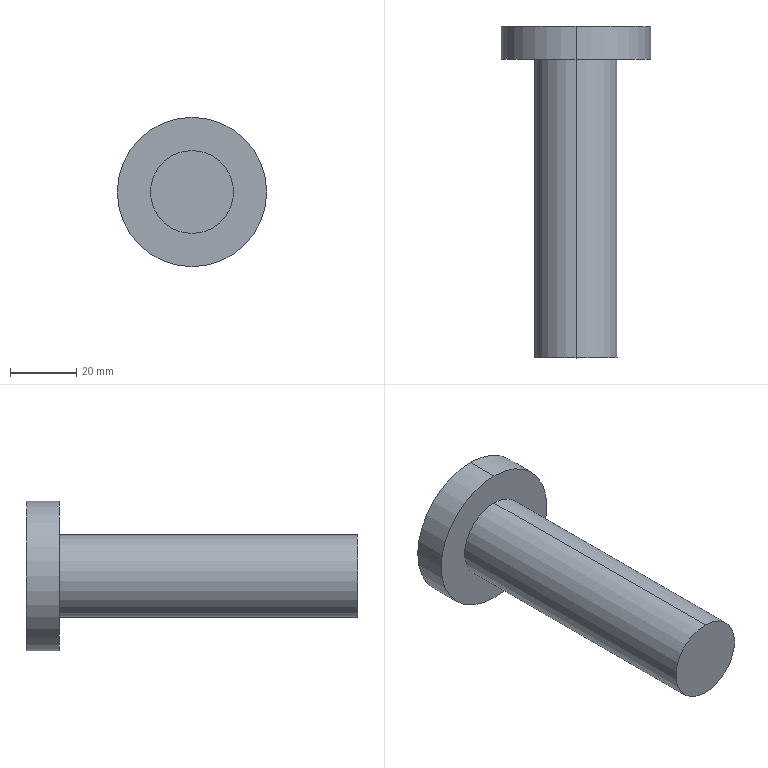Part | SolidWorks | features Extrusion 1, ICE 1 | 1 solid | 7 faces | box 45 x 100 x 45 mm | volume 60083 mm3 | cylinder 4 | plane 3 | commonest cylinder face diameters 25 x2 45 x2
STEP:
#1=CARTESIAN_POINT('',(0.,90.,22.5));
#2=VERTEX_POINT('',#1);
#3=CARTESIAN_POINT('',(0.,90.,-22.5));
#4=VERTEX_POINT('',#3);
#5=CARTESIAN_POINT('',(0.,90.,0.));
#6=DIRECTION('',(0.,1.,0.));
#7=DIRECTION('',(0.,0.,1.));
#8=AXIS2_PLACEMENT_3D('',#5,#6,#7);
#9=CIRCLE('',#8,22.5);
#10=EDGE_CURVE('',#2,#4,#9,.T.);
#11=ORIENTED_EDGE('',*,*,#10,.T.);
#12=CARTESIAN_POINT('',(0.,100.,-22.5));
#13=VERTEX_POINT('',#12);
#14=CARTESIAN_POINT('',(0.,90.,-22.5));
#15=DIRECTION('',(0.,1.,0.));
#16=VECTOR('',#15,1000.);
#17=LINE('',#14,#16);
#18=EDGE_CURVE('',#4,#13,#17,.T.);
#19=ORIENTED_EDGE('',*,*,#18,.T.);
#20=CARTESIAN_POINT('',(0.,100.,22.5));
#21=VERTEX_POINT('',#20);
#22=CARTESIAN_POINT('',(0.,100.,0.));
#23=DIRECTION('',(0.,1.,0.));
#24=DIRECTION('',(0.,0.,1.));
#25=AXIS2_PLACEMENT_3D('',#22,#23,#24);
#26=CIRCLE('',#25,22.5);
#27=EDGE_CURVE('',#21,#13,#26,.T.);
#28=ORIENTED_EDGE('',*,*,#27,.F.);
#29=CARTESIAN_POINT('',(0.,90.,22.5));
#30=DIRECTION('',(0.,1.,0.));
#31=VECTOR('',#30,1000.);
#32=LINE('',#29,#31);
#33=EDGE_CURVE('',#2,#21,#32,.T.);
#34=ORIENTED_EDGE('',*,*,#33,.F.);
#35=EDGE_LOOP('',(#11,#19,#28,#34));
#36=FACE_OUTER_BOUND('',#35,.T.);
#37=CARTESIAN_POINT('',(0.,90.,0.));
#38=DIRECTION('',(0.,1.,0.));
#39=DIRECTION('',(0.,0.,1.));
#40=AXIS2_PLACEMENT_3D('',#37,#38,#39);
#41=CYLINDRICAL_SURFACE('',#40,22.5);
#42=ADVANCED_FACE('',(#36),#41,.T.);
#43=CARTESIAN_POINT('',(0.,90.,12.5));
#44=VERTEX_POINT('',#43);
#45=CARTESIAN_POINT('',(0.,90.,-12.5));
#46=VERTEX_POINT('',#45);
#47=CARTESIAN_POINT('',(0.,90.,0.));
#48=DIRECTION('',(0.,1.,0.));
#49=DIRECTION('',(0.,0.,1.));
#50=AXIS2_PLACEMENT_3D('',#47,#48,#49);
#51=CIRCLE('',#50,12.5);
#52=EDGE_CURVE('',#44,#46,#51,.T.);
#53=ORIENTED_EDGE('',*,*,#52,.F.);
#54=CARTESIAN_POINT('',(0.,0.,12.5));
#55=VERTEX_POINT('',#54);
#56=CARTESIAN_POINT('',(0.,100.,12.5));
#57=DIRECTION('',(0.,-1.,0.));
#58=VECTOR('',#57,1000.);
#59=LINE('',#56,#58);
#60=EDGE_CURVE('',#44,#55,#59,.T.);
#61=ORIENTED_EDGE('',*,*,#60,.T.);
#62=CARTESIAN_POINT('',(0.,0.,-12.5));
#63=VERTEX_POINT('',#62);
#64=CARTESIAN_POINT('',(0.,0.,0.));
#65=DIRECTION('',(0.,1.,0.));
#66=DIRECTION('',(0.,0.,1.));
#67=AXIS2_PLACEMENT_3D('',#64,#65,#66);
#68=CIRCLE('',#67,12.5);
#69=EDGE_CURVE('',#55,#63,#68,.T.);
#70=ORIENTED_EDGE('',*,*,#69,.T.);
#71=CARTESIAN_POINT('',(0.,100.,-12.5));
#72=DIRECTION('',(0.,-1.,0.));
#73=VECTOR('',#72,1000.);
#74=LINE('',#71,#73);
#75=EDGE_CURVE('',#46,#63,#74,.T.);
#76=ORIENTED_EDGE('',*,*,#75,.F.);
#77=EDGE_LOOP('',(#53,#61,#70,#76));
#78=FACE_OUTER_BOUND('',#77,.T.);
#79=CARTESIAN_POINT('',(0.,100.,0.));
#80=DIRECTION('',(0.,-1.,0.));
#81=DIRECTION('',(0.,0.,-1.));
#82=AXIS2_PLACEMENT_3D('',#79,#80,#81);
#83=CYLINDRICAL_SURFACE('',#82,12.5);
#84=ADVANCED_FACE('',(#78),#83,.T.);
#85=ORIENTED_EDGE('',*,*,#60,.F.);
#86=CARTESIAN_POINT('',(0.,90.,0.));
#87=DIRECTION('',(0.,1.,0.));
#88=DIRECTION('',(0.,0.,1.));
#89=AXIS2_PLACEMENT_3D('',#86,#87,#88);
#90=CIRCLE('',#89,12.5);
#91=EDGE_CURVE('',#46,#44,#90,.T.);
#92=ORIENTED_EDGE('',*,*,#91,.F.);
#93=ORIENTED_EDGE('',*,*,#75,.T.);
#94=CARTESIAN_POINT('',(0.,0.,0.));
#95=DIRECTION('',(0.,1.,0.));
#96=DIRECTION('',(0.,0.,1.));
#97=AXIS2_PLACEMENT_3D('',#94,#95,#96);
#98=CIRCLE('',#97,12.5);
#99=EDGE_CURVE('',#63,#55,#98,.T.);
#100=ORIENTED_EDGE('',*,*,#99,.T.);
#101=EDGE_LOOP('',(#85,#92,#93,#100));
#102=FACE_OUTER_BOUND('',#101,.T.);
#103=CARTESIAN_POINT('',(0.,100.,0.));
#104=DIRECTION('',(0.,-1.,0.));
#105=DIRECTION('',(0.,0.,-1.));
#106=AXIS2_PLACEMENT_3D('',#103,#104,#105);
#107=CYLINDRICAL_SURFACE('',#106,12.5);
#108=ADVANCED_FACE('',(#102),#107,.T.);
#109=ORIENTED_EDGE('',*,*,#99,.F.);
#110=ORIENTED_EDGE('',*,*,#69,.F.);
#111=EDGE_LOOP('',(#109,#110));
#112=FACE_OUTER_BOUND('',#111,.T.);
#113=CARTESIAN_POINT('',(0.,0.,0.));
#114=DIRECTION('',(0.,1.,0.));
#115=DIRECTION('',(0.,0.,1.));
#116=AXIS2_PLACEMENT_3D('',#113,#114,#115);
#117=PLANE('',#116);
#118=ADVANCED_FACE('',(#112),#117,.F.);
#119=ORIENTED_EDGE('',*,*,#18,.F.);
#120=CARTESIAN_POINT('',(0.,90.,0.));
#121=DIRECTION('',(0.,1.,0.));
#122=DIRECTION('',(0.,0.,1.));
#123=AXIS2_PLACEMENT_3D('',#120,#121,#122);
#124=CIRCLE('',#123,22.5);
#125=EDGE_CURVE('',#4,#2,#124,.T.);
#126=ORIENTED_EDGE('',*,*,#125,.T.);
#127=ORIENTED_EDGE('',*,*,#33,.T.);
#128=CARTESIAN_POINT('',(0.,100.,0.));
#129=DIRECTION('',(0.,1.,0.));
#130=DIRECTION('',(0.,0.,1.));
#131=AXIS2_PLACEMENT_3D('',#128,#129,#130);
#132=CIRCLE('',#131,22.5);
#133=EDGE_CURVE('',#13,#21,#132,.T.);
#134=ORIENTED_EDGE('',*,*,#133,.F.);
#135=EDGE_LOOP('',(#119,#126,#127,#134));
#136=FACE_OUTER_BOUND('',#135,.T.);
#137=CARTESIAN_POINT('',(0.,90.,0.));
#138=DIRECTION('',(0.,1.,0.));
#139=DIRECTION('',(0.,0.,1.));
#140=AXIS2_PLACEMENT_3D('',#137,#138,#139);
#141=CYLINDRICAL_SURFACE('',#140,22.5);
#142=ADVANCED_FACE('',(#136),#141,.T.);
#143=ORIENTED_EDGE('',*,*,#91,.T.);
#144=ORIENTED_EDGE('',*,*,#52,.T.);
#145=EDGE_LOOP('',(#143,#144));
#146=FACE_BOUND('',#145,.T.);
#147=ORIENTED_EDGE('',*,*,#10,.F.);
#148=ORIENTED_EDGE('',*,*,#125,.F.);
#149=EDGE_LOOP('',(#147,#148));
#150=FACE_OUTER_BOUND('',#149,.T.);
#151=CARTESIAN_POINT('',(0.,90.,0.));
#152=DIRECTION('',(0.,1.,0.));
#153=DIRECTION('',(0.,0.,1.));
#154=AXIS2_PLACEMENT_3D('',#151,#152,#153);
#155=PLANE('',#154);
#156=ADVANCED_FACE('',(#146,#150),#155,.F.);
#157=ORIENTED_EDGE('',*,*,#27,.T.);
#158=ORIENTED_EDGE('',*,*,#133,.T.);
#159=EDGE_LOOP('',(#157,#158));
#160=FACE_OUTER_BOUND('',#159,.T.);
#161=CARTESIAN_POINT('',(0.,100.,0.));
#162=DIRECTION('',(0.,1.,0.));
#163=DIRECTION('',(0.,0.,1.));
#164=AXIS2_PLACEMENT_3D('',#161,#162,#163);
#165=PLANE('',#164);
#166=ADVANCED_FACE('',(#160),#165,.T.);
#167=CLOSED_SHELL('',(#42,#84,#108,#118,#142,#156,#166));
#168=MANIFOLD_SOLID_BREP('',#167);
#169=CARTESIAN_POINT('',(0.,0.,0.));
#170=DIRECTION('',(0.,0.,1.));
#171=DIRECTION('',(1.,0.,0.));
#172=AXIS2_PLACEMENT_3D('',#169,#170,#171);
#173=(LENGTH_UNIT()NAMED_UNIT(*)SI_UNIT(.MILLI.,.METRE.));
#174=UNCERTAINTY_MEASURE_WITH_UNIT(LENGTH_MEASURE(0.00001),#173,'','');
#175=(NAMED_UNIT(*)PLANE_ANGLE_UNIT()SI_UNIT($,.RADIAN.));
#176=(NAMED_UNIT(*)SI_UNIT($,.STERADIAN.)SOLID_ANGLE_UNIT());
#177=(GEOMETRIC_REPRESENTATION_CONTEXT(3)GLOBAL_UNCERTAINTY_ASSIGNED_CONTEXT((#174))GLOBAL_UNIT_ASSIGNED_CONTEXT((#173,#175,#176))REPRESENTATION_CONTEXT('',''));
#178=ADVANCED_BREP_SHAPE_REPRESENTATION('',(#168,#172),#177);